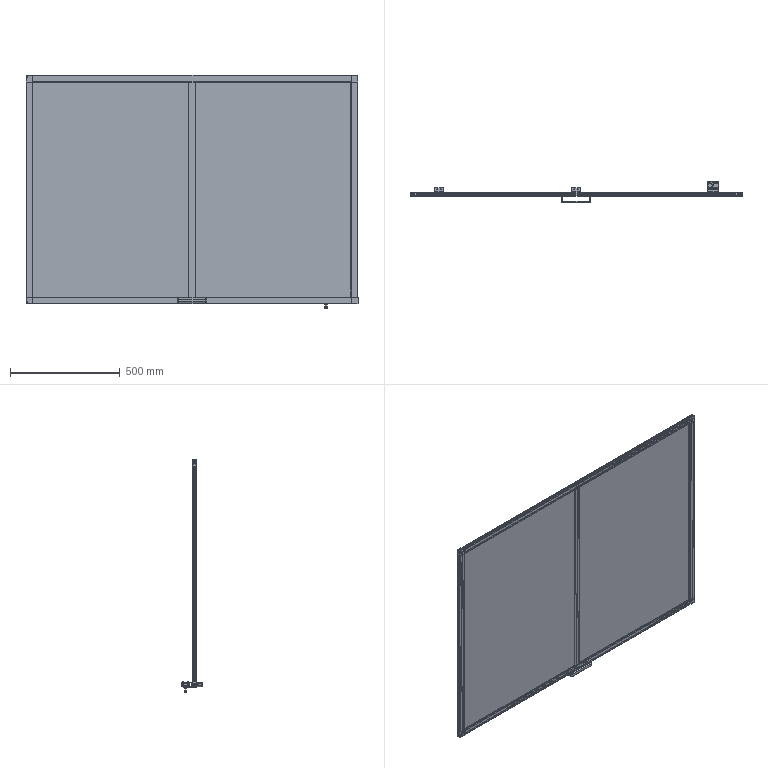Part | SolidWorks | features ReferencePattern 4, CompositeCurve 1, DerivedHolePattern 1, LocalLPattern 1 | 44 solids | 2289 faces | box 1516 x 97 x 1065 mm | volume 8783731 mm3 | plane 1101 | cylinder 591 | cone 370 | spline 128 | torus 87 | sphere 12 | commonest cylinder face diameters 1 x77 5 x72 11 x50 4.5 x48 3.3 x28 6.5 x28